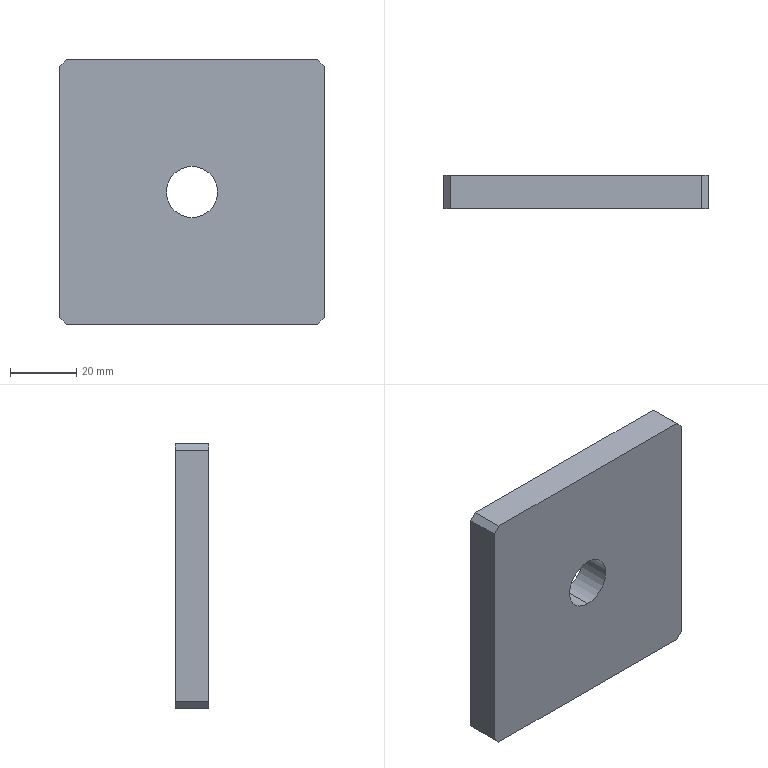Part | SolidWorks | features SplitBody 1 | 1 solid | 12 faces | box 80 x 10 x 80 mm | volume 62033 mm3 | plane 10 | cylinder 2 | commonest cylinder face diameters 15.5 x2
STEP:
#1=CARTESIAN_POINT('',(0.,-53.,267.75));
#2=VERTEX_POINT('',#1);
#3=CARTESIAN_POINT('',(0.,-53.,252.25));
#4=VERTEX_POINT('',#3);
#5=CARTESIAN_POINT('',(0.,-53.,260.));
#6=DIRECTION('',(0.,-1.,0.));
#7=DIRECTION('',(0.,0.,-1.));
#8=AXIS2_PLACEMENT_3D('',#5,#6,#7);
#9=CIRCLE('',#8,7.75);
#10=EDGE_CURVE('',#2,#4,#9,.T.);
#11=ORIENTED_EDGE('',*,*,#10,.F.);
#12=CARTESIAN_POINT('',(0.,-63.,267.75));
#13=VERTEX_POINT('',#12);
#14=CARTESIAN_POINT('',(0.,-53.,267.75));
#15=DIRECTION('',(0.,-1.,0.));
#16=VECTOR('',#15,1000.);
#17=LINE('',#14,#16);
#18=EDGE_CURVE('',#2,#13,#17,.T.);
#19=ORIENTED_EDGE('',*,*,#18,.T.);
#20=CARTESIAN_POINT('',(0.,-63.,252.25));
#21=VERTEX_POINT('',#20);
#22=CARTESIAN_POINT('',(0.,-63.,260.));
#23=DIRECTION('',(0.,-1.,0.));
#24=DIRECTION('',(0.,0.,-1.));
#25=AXIS2_PLACEMENT_3D('',#22,#23,#24);
#26=CIRCLE('',#25,7.75);
#27=EDGE_CURVE('',#13,#21,#26,.T.);
#28=ORIENTED_EDGE('',*,*,#27,.T.);
#29=CARTESIAN_POINT('',(0.,-53.,252.25));
#30=DIRECTION('',(0.,-1.,0.));
#31=VECTOR('',#30,1000.);
#32=LINE('',#29,#31);
#33=EDGE_CURVE('',#4,#21,#32,.T.);
#34=ORIENTED_EDGE('',*,*,#33,.F.);
#35=EDGE_LOOP('',(#11,#19,#28,#34));
#36=FACE_OUTER_BOUND('',#35,.T.);
#37=CARTESIAN_POINT('',(0.,-53.,260.));
#38=DIRECTION('',(0.,-1.,0.));
#39=DIRECTION('',(0.,0.,-1.));
#40=AXIS2_PLACEMENT_3D('',#37,#38,#39);
#41=CYLINDRICAL_SURFACE('',#40,7.75);
#42=ADVANCED_FACE('',(#36),#41,.F.);
#43=CARTESIAN_POINT('',(40.,-53.,222.));
#44=VERTEX_POINT('',#43);
#45=CARTESIAN_POINT('',(40.,-53.,298.));
#46=VERTEX_POINT('',#45);
#47=CARTESIAN_POINT('',(40.,-53.,300.));
#48=DIRECTION('',(0.,0.,1.));
#49=VECTOR('',#48,1000.);
#50=LINE('',#47,#49);
#51=EDGE_CURVE('',#44,#46,#50,.T.);
#52=ORIENTED_EDGE('',*,*,#51,.T.);
#53=CARTESIAN_POINT('',(40.,-63.,298.));
#54=VERTEX_POINT('',#53);
#55=CARTESIAN_POINT('',(40.,-63.,298.));
#56=DIRECTION('',(0.,-1.,0.));
#57=VECTOR('',#56,1000.);
#58=LINE('',#55,#57);
#59=EDGE_CURVE('',#46,#54,#58,.T.);
#60=ORIENTED_EDGE('',*,*,#59,.T.);
#61=CARTESIAN_POINT('',(40.,-63.,222.));
#62=VERTEX_POINT('',#61);
#63=CARTESIAN_POINT('',(40.,-63.,300.));
#64=DIRECTION('',(0.,0.,1.));
#65=VECTOR('',#64,1000.);
#66=LINE('',#63,#65);
#67=EDGE_CURVE('',#62,#54,#66,.T.);
#68=ORIENTED_EDGE('',*,*,#67,.F.);
#69=CARTESIAN_POINT('',(40.,-63.,222.));
#70=DIRECTION('',(0.,1.,0.));
#71=VECTOR('',#70,1000.);
#72=LINE('',#69,#71);
#73=EDGE_CURVE('',#62,#44,#72,.T.);
#74=ORIENTED_EDGE('',*,*,#73,.T.);
#75=EDGE_LOOP('',(#52,#60,#68,#74));
#76=FACE_OUTER_BOUND('',#75,.T.);
#77=CARTESIAN_POINT('',(40.,-63.,300.));
#78=DIRECTION('',(-1.,0.,0.));
#79=DIRECTION('',(0.,0.,1.));
#80=AXIS2_PLACEMENT_3D('',#77,#78,#79);
#81=PLANE('',#80);
#82=ADVANCED_FACE('',(#76),#81,.F.);
#83=CARTESIAN_POINT('',(38.,-63.,300.));
#84=VERTEX_POINT('',#83);
#85=CARTESIAN_POINT('',(-38.,-63.,300.));
#86=VERTEX_POINT('',#85);
#87=CARTESIAN_POINT('',(-40.,-63.,300.));
#88=DIRECTION('',(-1.,0.,0.));
#89=VECTOR('',#88,1000.);
#90=LINE('',#87,#89);
#91=EDGE_CURVE('',#84,#86,#90,.T.);
#92=ORIENTED_EDGE('',*,*,#91,.F.);
#93=CARTESIAN_POINT('',(38.,-53.,300.));
#94=VERTEX_POINT('',#93);
#95=CARTESIAN_POINT('',(38.,-63.,300.));
#96=DIRECTION('',(0.,1.,0.));
#97=VECTOR('',#96,1000.);
#98=LINE('',#95,#97);
#99=EDGE_CURVE('',#84,#94,#98,.T.);
#100=ORIENTED_EDGE('',*,*,#99,.T.);
#101=CARTESIAN_POINT('',(-38.,-53.,300.));
#102=VERTEX_POINT('',#101);
#103=CARTESIAN_POINT('',(-40.,-53.,300.));
#104=DIRECTION('',(-1.,0.,0.));
#105=VECTOR('',#104,1000.);
#106=LINE('',#103,#105);
#107=EDGE_CURVE('',#94,#102,#106,.T.);
#108=ORIENTED_EDGE('',*,*,#107,.T.);
#109=CARTESIAN_POINT('',(-38.,-63.,300.));
#110=DIRECTION('',(0.,-1.,0.));
#111=VECTOR('',#110,1000.);
#112=LINE('',#109,#111);
#113=EDGE_CURVE('',#102,#86,#112,.T.);
#114=ORIENTED_EDGE('',*,*,#113,.T.);
#115=EDGE_LOOP('',(#92,#100,#108,#114));
#116=FACE_OUTER_BOUND('',#115,.T.);
#117=CARTESIAN_POINT('',(-40.,-63.,300.));
#118=DIRECTION('',(0.,0.,-1.));
#119=DIRECTION('',(0.,1.,0.));
#120=AXIS2_PLACEMENT_3D('',#117,#118,#119);
#121=PLANE('',#120);
#122=ADVANCED_FACE('',(#116),#121,.F.);
#123=CARTESIAN_POINT('',(-40.,-53.,298.));
#124=VERTEX_POINT('',#123);
#125=CARTESIAN_POINT('',(-40.,-53.,222.));
#126=VERTEX_POINT('',#125);
#127=CARTESIAN_POINT('',(-40.,-53.,300.));
#128=DIRECTION('',(0.,0.,-1.));
#129=VECTOR('',#128,1000.);
#130=LINE('',#127,#129);
#131=EDGE_CURVE('',#124,#126,#130,.T.);
#132=ORIENTED_EDGE('',*,*,#131,.T.);
#133=CARTESIAN_POINT('',(-40.,-63.,222.));
#134=VERTEX_POINT('',#133);
#135=CARTESIAN_POINT('',(-40.,-63.,222.));
#136=DIRECTION('',(0.,-1.,0.));
#137=VECTOR('',#136,1000.);
#138=LINE('',#135,#137);
#139=EDGE_CURVE('',#126,#134,#138,.T.);
#140=ORIENTED_EDGE('',*,*,#139,.T.);
#141=CARTESIAN_POINT('',(-40.,-63.,298.));
#142=VERTEX_POINT('',#141);
#143=CARTESIAN_POINT('',(-40.,-63.,300.));
#144=DIRECTION('',(0.,0.,-1.));
#145=VECTOR('',#144,1000.);
#146=LINE('',#143,#145);
#147=EDGE_CURVE('',#142,#134,#146,.T.);
#148=ORIENTED_EDGE('',*,*,#147,.F.);
#149=CARTESIAN_POINT('',(-40.,-63.,298.));
#150=DIRECTION('',(0.,1.,0.));
#151=VECTOR('',#150,1000.);
#152=LINE('',#149,#151);
#153=EDGE_CURVE('',#142,#124,#152,.T.);
#154=ORIENTED_EDGE('',*,*,#153,.T.);
#155=EDGE_LOOP('',(#132,#140,#148,#154));
#156=FACE_OUTER_BOUND('',#155,.T.);
#157=CARTESIAN_POINT('',(-40.,-63.,300.));
#158=DIRECTION('',(1.,0.,0.));
#159=DIRECTION('',(0.,0.,-1.));
#160=AXIS2_PLACEMENT_3D('',#157,#158,#159);
#161=PLANE('',#160);
#162=ADVANCED_FACE('',(#156),#161,.F.);
#163=CARTESIAN_POINT('',(-38.,-53.,220.));
#164=VERTEX_POINT('',#163);
#165=CARTESIAN_POINT('',(38.,-53.,220.));
#166=VERTEX_POINT('',#165);
#167=CARTESIAN_POINT('',(-40.,-53.,220.));
#168=DIRECTION('',(1.,0.,0.));
#169=VECTOR('',#168,1000.);
#170=LINE('',#167,#169);
#171=EDGE_CURVE('',#164,#166,#170,.T.);
#172=ORIENTED_EDGE('',*,*,#171,.T.);
#173=CARTESIAN_POINT('',(38.,-63.,220.));
#174=VERTEX_POINT('',#173);
#175=CARTESIAN_POINT('',(38.,-63.,220.));
#176=DIRECTION('',(0.,-1.,0.));
#177=VECTOR('',#176,1000.);
#178=LINE('',#175,#177);
#179=EDGE_CURVE('',#166,#174,#178,.T.);
#180=ORIENTED_EDGE('',*,*,#179,.T.);
#181=CARTESIAN_POINT('',(-38.,-63.,220.));
#182=VERTEX_POINT('',#181);
#183=CARTESIAN_POINT('',(-40.,-63.,220.));
#184=DIRECTION('',(1.,0.,0.));
#185=VECTOR('',#184,1000.);
#186=LINE('',#183,#185);
#187=EDGE_CURVE('',#182,#174,#186,.T.);
#188=ORIENTED_EDGE('',*,*,#187,.F.);
#189=CARTESIAN_POINT('',(-38.,-63.,220.));
#190=DIRECTION('',(0.,1.,0.));
#191=VECTOR('',#190,1000.);
#192=LINE('',#189,#191);
#193=EDGE_CURVE('',#182,#164,#192,.T.);
#194=ORIENTED_EDGE('',*,*,#193,.T.);
#195=EDGE_LOOP('',(#172,#180,#188,#194));
#196=FACE_OUTER_BOUND('',#195,.T.);
#197=CARTESIAN_POINT('',(-40.,-63.,220.));
#198=DIRECTION('',(0.,0.,1.));
#199=DIRECTION('',(0.,-1.,0.));
#200=AXIS2_PLACEMENT_3D('',#197,#198,#199);
#201=PLANE('',#200);
#202=ADVANCED_FACE('',(#196),#201,.F.);
#203=CARTESIAN_POINT('',(0.,-63.,260.));
#204=DIRECTION('',(0.,-1.,0.));
#205=DIRECTION('',(0.,0.,-1.));
#206=AXIS2_PLACEMENT_3D('',#203,#204,#205);
#207=CIRCLE('',#206,7.75);
#208=EDGE_CURVE('',#21,#13,#207,.T.);
#209=ORIENTED_EDGE('',*,*,#208,.F.);
#210=ORIENTED_EDGE('',*,*,#27,.F.);
#211=EDGE_LOOP('',(#209,#210));
#212=FACE_BOUND('',#211,.T.);
#213=ORIENTED_EDGE('',*,*,#67,.T.);
#214=CARTESIAN_POINT('',(169.,-63.,169.));
#215=DIRECTION('',(-0.7071,0.,0.7071));
#216=VECTOR('',#215,1000.);
#217=LINE('',#214,#216);
#218=EDGE_CURVE('',#54,#84,#217,.T.);
#219=ORIENTED_EDGE('',*,*,#218,.T.);
#220=ORIENTED_EDGE('',*,*,#91,.T.);
#221=CARTESIAN_POINT('',(-169.,-63.,169.));
#222=DIRECTION('',(-0.7071,0.,-0.7071));
#223=VECTOR('',#222,1000.);
#224=LINE('',#221,#223);
#225=EDGE_CURVE('',#86,#142,#224,.T.);
#226=ORIENTED_EDGE('',*,*,#225,.T.);
#227=ORIENTED_EDGE('',*,*,#147,.T.);
#228=CARTESIAN_POINT('',(91.,-63.,91.));
#229=DIRECTION('',(0.7071,0.,-0.7071));
#230=VECTOR('',#229,1000.);
#231=LINE('',#228,#230);
#232=EDGE_CURVE('',#134,#182,#231,.T.);
#233=ORIENTED_EDGE('',*,*,#232,.T.);
#234=ORIENTED_EDGE('',*,*,#187,.T.);
#235=CARTESIAN_POINT('',(-91.,-63.,91.));
#236=DIRECTION('',(0.7071,0.,0.7071));
#237=VECTOR('',#236,1000.);
#238=LINE('',#235,#237);
#239=EDGE_CURVE('',#174,#62,#238,.T.);
#240=ORIENTED_EDGE('',*,*,#239,.T.);
#241=EDGE_LOOP('',(#213,#219,#220,#226,#227,#233,#234,#240));
#242=FACE_OUTER_BOUND('',#241,.T.);
#243=CARTESIAN_POINT('',(0.,-63.,0.));
#244=DIRECTION('',(0.,-1.,0.));
#245=DIRECTION('',(0.,0.,-1.));
#246=AXIS2_PLACEMENT_3D('',#243,#244,#245);
#247=PLANE('',#246);
#248=ADVANCED_FACE('',(#212,#242),#247,.T.);
#249=CARTESIAN_POINT('',(0.,-53.,260.));
#250=DIRECTION('',(0.,-1.,0.));
#251=DIRECTION('',(0.,0.,-1.));
#252=AXIS2_PLACEMENT_3D('',#249,#250,#251);
#253=CIRCLE('',#252,7.75);
#254=EDGE_CURVE('',#4,#2,#253,.T.);
#255=ORIENTED_EDGE('',*,*,#254,.T.);
#256=ORIENTED_EDGE('',*,*,#10,.T.);
#257=EDGE_LOOP('',(#255,#256));
#258=FACE_BOUND('',#257,.T.);
#259=ORIENTED_EDGE('',*,*,#107,.F.);
#260=CARTESIAN_POINT('',(38.,-53.,300.));
#261=DIRECTION('',(0.7071,0.,-0.7071));
#262=VECTOR('',#261,1000.);
#263=LINE('',#260,#262);
#264=EDGE_CURVE('',#94,#46,#263,.T.);
#265=ORIENTED_EDGE('',*,*,#264,.T.);
#266=ORIENTED_EDGE('',*,*,#51,.F.);
#267=CARTESIAN_POINT('',(40.,-53.,222.));
#268=DIRECTION('',(-0.7071,0.,-0.7071));
#269=VECTOR('',#268,1000.);
#270=LINE('',#267,#269);
#271=EDGE_CURVE('',#44,#166,#270,.T.);
#272=ORIENTED_EDGE('',*,*,#271,.T.);
#273=ORIENTED_EDGE('',*,*,#171,.F.);
#274=CARTESIAN_POINT('',(-38.,-53.,220.));
#275=DIRECTION('',(-0.7071,0.,0.7071));
#276=VECTOR('',#275,1000.);
#277=LINE('',#274,#276);
#278=EDGE_CURVE('',#164,#126,#277,.T.);
#279=ORIENTED_EDGE('',*,*,#278,.T.);
#280=ORIENTED_EDGE('',*,*,#131,.F.);
#281=CARTESIAN_POINT('',(-40.,-53.,298.));
#282=DIRECTION('',(0.7071,0.,0.7071));
#283=VECTOR('',#282,1000.);
#284=LINE('',#281,#283);
#285=EDGE_CURVE('',#124,#102,#284,.T.);
#286=ORIENTED_EDGE('',*,*,#285,.T.);
#287=EDGE_LOOP('',(#259,#265,#266,#272,#273,#279,#280,#286));
#288=FACE_OUTER_BOUND('',#287,.T.);
#289=CARTESIAN_POINT('',(0.,-53.,0.));
#290=DIRECTION('',(0.,-1.,0.));
#291=DIRECTION('',(0.,0.,-1.));
#292=AXIS2_PLACEMENT_3D('',#289,#290,#291);
#293=PLANE('',#292);
#294=ADVANCED_FACE('',(#258,#288),#293,.F.);
#295=ORIENTED_EDGE('',*,*,#18,.F.);
#296=ORIENTED_EDGE('',*,*,#254,.F.);
#297=ORIENTED_EDGE('',*,*,#33,.T.);
#298=ORIENTED_EDGE('',*,*,#208,.T.);
#299=EDGE_LOOP('',(#295,#296,#297,#298));
#300=FACE_OUTER_BOUND('',#299,.T.);
#301=CARTESIAN_POINT('',(0.,-53.,260.));
#302=DIRECTION('',(0.,-1.,0.));
#303=DIRECTION('',(0.,0.,-1.));
#304=AXIS2_PLACEMENT_3D('',#301,#302,#303);
#305=CYLINDRICAL_SURFACE('',#304,7.75);
#306=ADVANCED_FACE('',(#300),#305,.F.);
#307=ORIENTED_EDGE('',*,*,#218,.F.);
#308=ORIENTED_EDGE('',*,*,#59,.F.);
#309=ORIENTED_EDGE('',*,*,#264,.F.);
#310=ORIENTED_EDGE('',*,*,#99,.F.);
#311=EDGE_LOOP('',(#307,#308,#309,#310));
#312=FACE_OUTER_BOUND('',#311,.T.);
#313=CARTESIAN_POINT('',(38.,-63.,300.));
#314=DIRECTION('',(-0.7071,0.,-0.7071));
#315=DIRECTION('',(0.,1.,0.));
#316=AXIS2_PLACEMENT_3D('',#313,#314,#315);
#317=PLANE('',#316);
#318=ADVANCED_FACE('',(#312),#317,.F.);
#319=ORIENTED_EDGE('',*,*,#239,.F.);
#320=ORIENTED_EDGE('',*,*,#179,.F.);
#321=ORIENTED_EDGE('',*,*,#271,.F.);
#322=ORIENTED_EDGE('',*,*,#73,.F.);
#323=EDGE_LOOP('',(#319,#320,#321,#322));
#324=FACE_OUTER_BOUND('',#323,.T.);
#325=CARTESIAN_POINT('',(40.,-63.,222.));
#326=DIRECTION('',(-0.7071,0.,0.7071));
#327=DIRECTION('',(0.,1.,0.));
#328=AXIS2_PLACEMENT_3D('',#325,#326,#327);
#329=PLANE('',#328);
#330=ADVANCED_FACE('',(#324),#329,.F.);
#331=ORIENTED_EDGE('',*,*,#232,.F.);
#332=ORIENTED_EDGE('',*,*,#139,.F.);
#333=ORIENTED_EDGE('',*,*,#278,.F.);
#334=ORIENTED_EDGE('',*,*,#193,.F.);
#335=EDGE_LOOP('',(#331,#332,#333,#334));
#336=FACE_OUTER_BOUND('',#335,.T.);
#337=CARTESIAN_POINT('',(-38.,-63.,220.));
#338=DIRECTION('',(0.7071,0.,0.7071));
#339=DIRECTION('',(0.,1.,0.));
#340=AXIS2_PLACEMENT_3D('',#337,#338,#339);
#341=PLANE('',#340);
#342=ADVANCED_FACE('',(#336),#341,.F.);
#343=ORIENTED_EDGE('',*,*,#225,.F.);
#344=ORIENTED_EDGE('',*,*,#113,.F.);
#345=ORIENTED_EDGE('',*,*,#285,.F.);
#346=ORIENTED_EDGE('',*,*,#153,.F.);
#347=EDGE_LOOP('',(#343,#344,#345,#346));
#348=FACE_OUTER_BOUND('',#347,.T.);
#349=CARTESIAN_POINT('',(-40.,-63.,298.));
#350=DIRECTION('',(0.7071,0.,-0.7071));
#351=DIRECTION('',(0.,1.,0.));
#352=AXIS2_PLACEMENT_3D('',#349,#350,#351);
#353=PLANE('',#352);
#354=ADVANCED_FACE('',(#348),#353,.F.);
#355=CLOSED_SHELL('',(#42,#82,#122,#162,#202,#248,#294,#306,#318,#330,#342,#354));
#356=MANIFOLD_SOLID_BREP('',#355);
#357=CARTESIAN_POINT('',(0.,0.,0.));
#358=DIRECTION('',(0.,0.,1.));
#359=DIRECTION('',(1.,0.,0.));
#360=AXIS2_PLACEMENT_3D('',#357,#358,#359);
#361=(LENGTH_UNIT()NAMED_UNIT(*)SI_UNIT(.MILLI.,.METRE.));
#362=UNCERTAINTY_MEASURE_WITH_UNIT(LENGTH_MEASURE(0.00001),#361,'','');
#363=(NAMED_UNIT(*)PLANE_ANGLE_UNIT()SI_UNIT($,.RADIAN.));
#364=(NAMED_UNIT(*)SI_UNIT($,.STERADIAN.)SOLID_ANGLE_UNIT());
#365=(GEOMETRIC_REPRESENTATION_CONTEXT(3)GLOBAL_UNCERTAINTY_ASSIGNED_CONTEXT((#362))GLOBAL_UNIT_ASSIGNED_CONTEXT((#361,#363,#364))REPRESENTATION_CONTEXT('',''));
#366=ADVANCED_BREP_SHAPE_REPRESENTATION('',(#356,#360),#365);